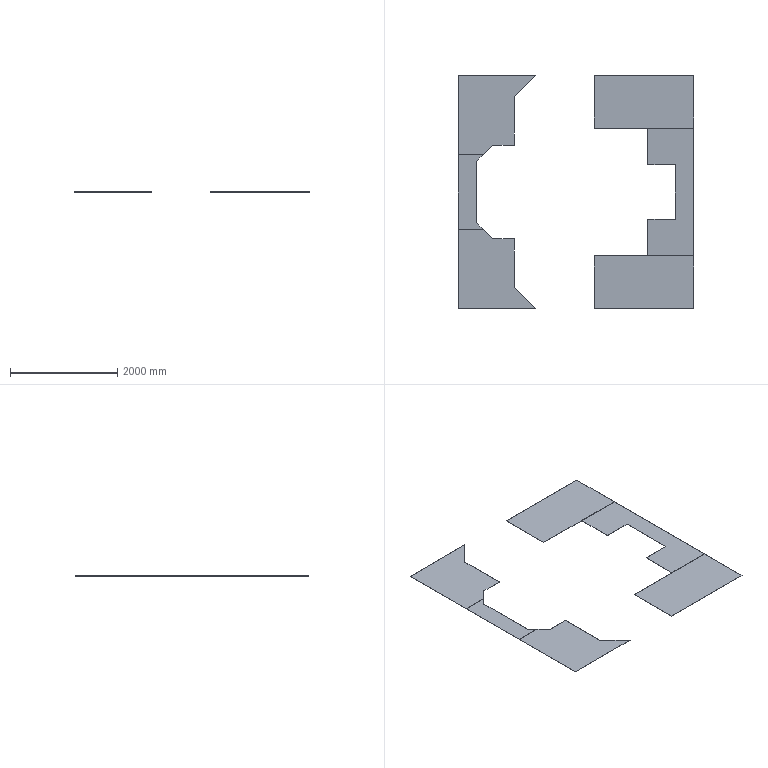Part | STEP file | 计量花纹Plate | 6 solids | 48 faces | box 4394 x 4350 x 3 mm | volume 26297241 mm3 | plane 48